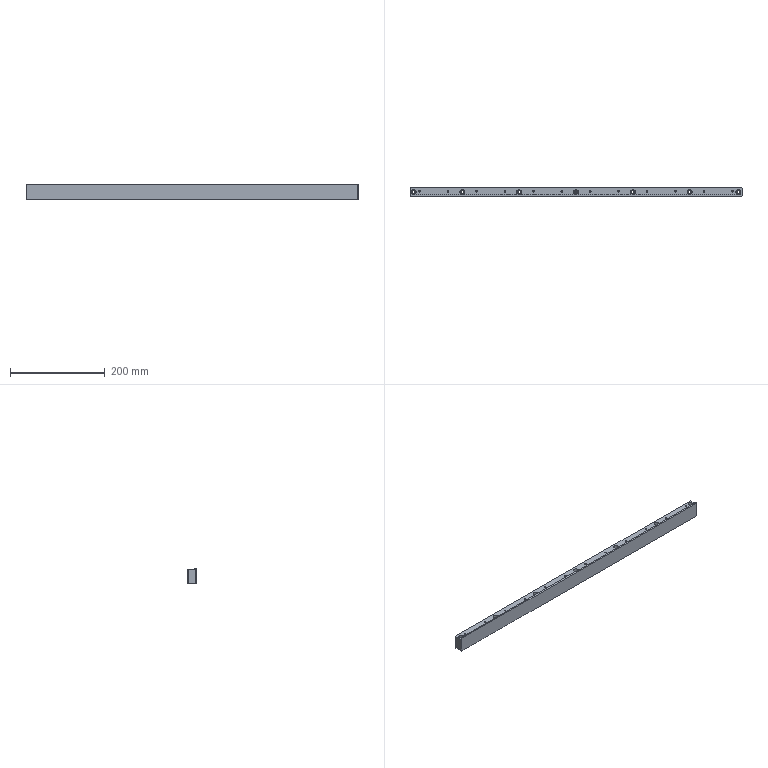Part | SolidWorks | features HoleWzd 3, Chamfer 1, Extrusion 1, ICE 1 | 1 solid | 103 faces | box 700 x 18 x 33 mm | volume 370685 mm3 | cylinder 56 | cone 28 | plane 19 | commonest cylinder face diameters 3.3 x24 5.5 x14 10 x14 8 x4